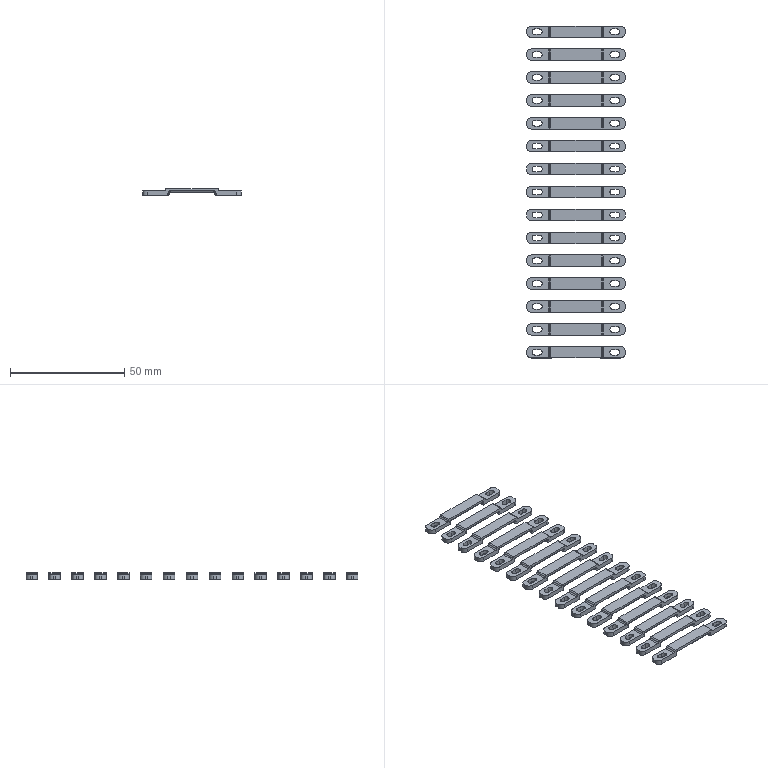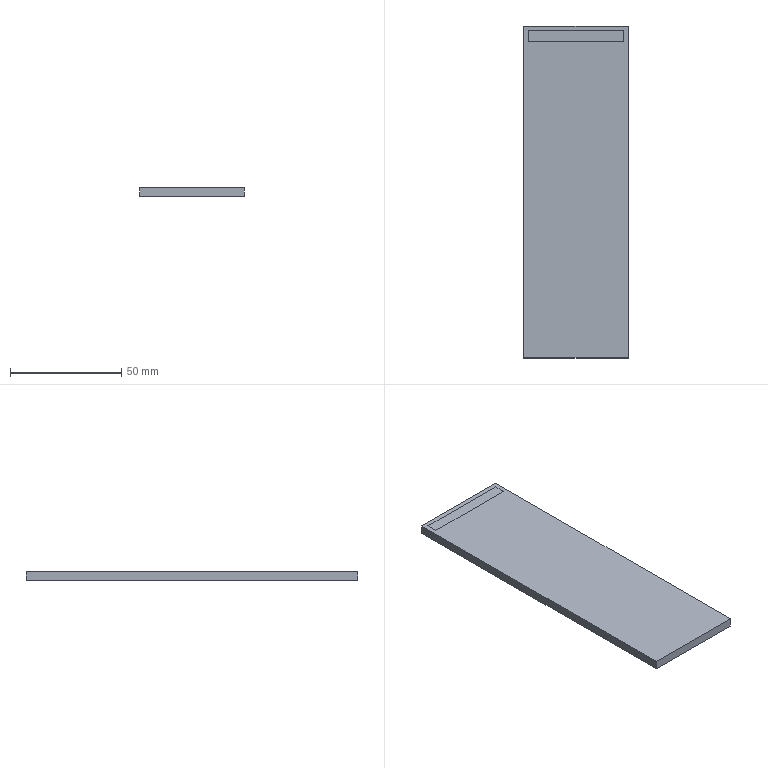CAM job | NX | 3-axis milling | part box 43 x 145 x 3 mm | stock box 47 x 149 x 4 mm
Tools:
number,name,description,diameter,corner_radius,flute_length,length,flutes
19,D80,Milling Tool-5 Parameters,80.0,0.0,50.0,75.0,2
11,D4,Milling Tool-5 Parameters,4.0,0.0,50.0,75.0,2
17,D2,Milling Tool-5 Parameters,2.0,0.0,50.0,75.0,2
16,D2R0.5,Milling Tool-5 Parameters,2.0,0.5,50.0,75.0,2
1,D6A45,Milling Tool-5 Parameters,6.0,0.0,50.0,75.0,2
15,D10JING,Milling Tool-5 Parameters,10.0,0.0,50.0,75.0,2
Operations:
program,operation,operation_type,tool,method,geometry_group,spindle_rpm,surface_speed,feed_per_tooth,feed_cut,feed_plunge,cut_length_mm,path_length_mm,cut_time_min,machine_time_min
1,FLOOR_WALL,VolumeBased25DMillingOperation,D80,METHOD,A,6500.0,1633.0,0.1154,1500.0,100.0,241.0,295.0,0.1607,0.1661
1,ZLEVEL_PROFILE,ZLevelMilling,D4,METHOD,A,9500.0,119.0,0.1316,2500.0,1000.0,10429.556,11855.378,4.499,4.641
1,FLOOR_WALL_1,VolumeBased25DMillingOperation,D4,METHOD,A,9500.0,119.0,0.1316,2500.0,1000.0,5718.875,10536.632,2.41,2.891
1,FLOOR_WALL_1_COPY,VolumeBased25DMillingOperation,D4,METHOD,A,9500.0,119.0,0.0789,1500.0,1000.0,1372.534,2485.92,0.9254,1.037
1,PLANAR_MILL_COPY_COPY_COPY_COPY_COPY_COPY_1,PlanarMilling,D6A45,METHOD,A,9500.0,179.0,0.0658,1250.0,100.0,1577.592,5549.332,1.262,1.659
1,ZLEVEL_PROFILE_COPY,ZLevelMilling,D2,METHOD,A,18939.0,119.0,0.0317,1200.0,1000.0,2107.924,4253.288,1.823,2.038
1,ZLEVEL_PROFILE_COPY_COPY,ZLevelMilling,D2R0.5,METHOD,A,9500.0,59.0,0.1316,2500.0,1000.0,340.517,482.4,0.1381,0.1523
1,ZLEVEL_PROFILE_COPY_COPY_COPY,ZLevelMilling,D2R0.5,METHOD,A,9500.0,59.0,0.1316,2500.0,1000.0,573.496,704.599,0.2312,0.2443
1,ZLEVEL_PROFILE_COPY_COPY_COPY_1,ZLevelMilling,D2R0.5,METHOD,A,9500.0,59.0,0.1316,2500.0,1000.0,340.517,482.4,0.1381,0.1523
1,ZLEVEL_PROFILE_COPY_COPY_COPY_COPY,ZLevelMilling,D2R0.5,METHOD,A,9500.0,59.0,0.1316,2500.0,1000.0,573.496,704.599,0.2312,0.2443
1,ZLEVEL_PROFILE_COPY_COPY_COPY_2,ZLevelMilling,D2R0.5,METHOD,A,9500.0,59.0,0.1316,2500.0,1000.0,340.517,482.4,0.1381,0.1523
1,ZLEVEL_PROFILE_COPY_COPY_COPY_COPY_1,ZLevelMilling,D2R0.5,METHOD,A,9500.0,59.0,0.1316,2500.0,1000.0,573.496,704.599,0.2312,0.2443
1,ZLEVEL_PROFILE_COPY_COPY_COPY_3,ZLevelMilling,D2R0.5,METHOD,A,9500.0,59.0,0.1316,2500.0,1000.0,340.517,482.4,0.1381,0.1523
1,ZLEVEL_PROFILE_COPY_COPY_COPY_COPY_2,ZLevelMilling,D2R0.5,METHOD,A,9500.0,59.0,0.1316,2500.0,1000.0,573.496,704.599,0.2312,0.2443
1,ZLEVEL_PROFILE_COPY_COPY_COPY_4,ZLevelMilling,D2R0.5,METHOD,A,9500.0,59.0,0.1316,2500.0,1000.0,340.517,482.4,0.1381,0.1523
1,ZLEVEL_PROFILE_COPY_COPY_COPY_COPY_3,ZLevelMilling,D2R0.5,METHOD,A,9500.0,59.0,0.1316,2500.0,1000.0,573.496,704.599,0.2312,0.2443
1,ZLEVEL_PROFILE_COPY_COPY_COPY_5,ZLevelMilling,D2R0.5,METHOD,A,9500.0,59.0,0.1316,2500.0,1000.0,340.517,482.4,0.1381,0.1523
1,ZLEVEL_PROFILE_COPY_COPY_COPY_COPY_4,ZLevelMilling,D2R0.5,METHOD,A,9500.0,59.0,0.1316,2500.0,1000.0,573.496,704.599,0.2312,0.2443
1,ZLEVEL_PROFILE_COPY_COPY_COPY_6,ZLevelMilling,D2R0.5,METHOD,A,9500.0,59.0,0.1316,2500.0,1000.0,340.517,482.4,0.1381,0.1523
1,ZLEVEL_PROFILE_COPY_COPY_COPY_COPY_5,ZLevelMilling,D2R0.5,METHOD,A,9500.0,59.0,0.1316,2500.0,1000.0,573.496,704.599,0.2312,0.2443
1,ZLEVEL_PROFILE_COPY_COPY_COPY_7,ZLevelMilling,D2R0.5,METHOD,A,9500.0,59.0,0.1316,2500.0,1000.0,340.517,482.4,0.1381,0.1523
1,ZLEVEL_PROFILE_COPY_COPY_COPY_COPY_6,ZLevelMilling,D2R0.5,METHOD,A,9500.0,59.0,0.1316,2500.0,1000.0,573.496,704.599,0.2312,0.2443
1,ZLEVEL_PROFILE_COPY_COPY_COPY_8,ZLevelMilling,D2R0.5,METHOD,A,9500.0,59.0,0.1316,2500.0,1000.0,340.517,482.4,0.1381,0.1523
1,ZLEVEL_PROFILE_COPY_COPY_COPY_COPY_7,ZLevelMilling,D2R0.5,METHOD,A,9500.0,59.0,0.1316,2500.0,1000.0,573.496,704.599,0.2312,0.2443
1,ZLEVEL_PROFILE_COPY_COPY_COPY_9,ZLevelMilling,D2R0.5,METHOD,A,9500.0,59.0,0.1316,2500.0,1000.0,340.517,482.4,0.1381,0.1523
1,ZLEVEL_PROFILE_COPY_COPY_COPY_COPY_8,ZLevelMilling,D2R0.5,METHOD,A,9500.0,59.0,0.1316,2500.0,1000.0,573.496,704.599,0.2312,0.2443
1,ZLEVEL_PROFILE_COPY_COPY_COPY_10,ZLevelMilling,D2R0.5,METHOD,A,9500.0,59.0,0.1316,2500.0,1000.0,340.517,482.4,0.1381,0.1523
1,ZLEVEL_PROFILE_COPY_COPY_COPY_COPY_9,ZLevelMilling,D2R0.5,METHOD,A,9500.0,59.0,0.1316,2500.0,1000.0,573.496,704.599,0.2312,0.2443
1,ZLEVEL_PROFILE_COPY_COPY_COPY_11,ZLevelMilling,D2R0.5,METHOD,A,9500.0,59.0,0.1316,2500.0,1000.0,340.517,482.4,0.1381,0.1523
1,ZLEVEL_PROFILE_COPY_COPY_COPY_COPY_10,ZLevelMilling,D2R0.5,METHOD,A,9500.0,59.0,0.1316,2500.0,1000.0,573.496,704.599,0.2312,0.2443
1,ZLEVEL_PROFILE_COPY_COPY_COPY_12,ZLevelMilling,D2R0.5,METHOD,A,9500.0,59.0,0.1316,2500.0,1000.0,340.517,482.4,0.1381,0.1523
1,ZLEVEL_PROFILE_COPY_COPY_COPY_COPY_11,ZLevelMilling,D2R0.5,METHOD,A,9500.0,59.0,0.1316,2500.0,1000.0,573.496,704.599,0.2312,0.2443
1,ZLEVEL_PROFILE_COPY_COPY_COPY_13,ZLevelMilling,D2R0.5,METHOD,A,9500.0,59.0,0.1316,2500.0,1000.0,340.517,482.4,0.1381,0.1523
1,ZLEVEL_PROFILE_COPY_COPY_COPY_COPY_12,ZLevelMilling,D2R0.5,METHOD,A,9500.0,59.0,0.1316,2500.0,1000.0,573.496,704.599,0.2312,0.2443
1,ZLEVEL_PROFILE_COPY_COPY_COPY_14,ZLevelMilling,D2R0.5,METHOD,A,9500.0,59.0,0.1316,2500.0,1000.0,340.517,482.4,0.1381,0.1523
1,ZLEVEL_PROFILE_COPY_COPY_COPY_COPY_13,ZLevelMilling,D2R0.5,METHOD,A,9500.0,59.0,0.1316,2500.0,1000.0,573.496,704.599,0.2312,0.2443
1,ZLEVEL_PROFILE_COPY_1,ZLevelMilling,D4,METHOD,A,9500.0,119.0,0.0632,1200.0,1000.0,6478.31,8340.265,5.405,5.591
2,FLOOR_WALL_COPY,VolumeBased25DMillingOperation,D10JING,METHOD,B,6500.0,1633.0,0.1154,1500.0,100.0,65.0,119.0,0.0433,0.0487
2,FLOOR_WALL_1_COPY_1,VolumeBased25DMillingOperation,D4,METHOD,B,9500.0,119.0,0.1316,2500.0,1000.0,431.469,908.78,0.19,0.2377
2,FLOOR_WALL_1_COPY_COPY,VolumeBased25DMillingOperation,D4,METHOD,B,9500.0,119.0,0.0789,1500.0,1000.0,122.724,282.711,0.0834,0.0994
2,ZLEVEL_PROFILE_COPY_COPY_COPY_15,ZLevelMilling,D2R0.5,METHOD,B,9500.0,59.0,0.1316,2500.0,1000.0,158.516,301.495,0.0652,0.0795
2,PLANAR_MILL_COPY_COPY_COPY_COPY_COPY_COPY_1_COPY,PlanarMilling,D6A45,METHOD,B,9500.0,179.0,0.0658,1250.0,100.0,54.189,179.989,0.0434,0.0559
2,PLANAR_MILL_COPY_COPY_COPY_COPY_COPY_COPY_1_COPY_COPY,PlanarMilling,D6A45,METHOD,B,9500.0,179.0,0.0658,1250.0,100.0,86.419,364.989,0.0691,0.097